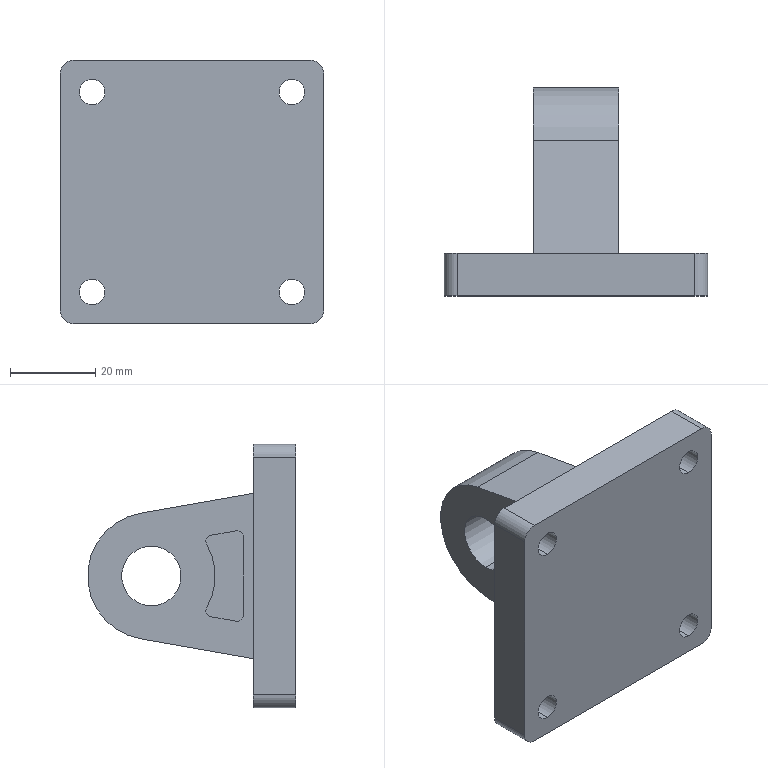Part | STEP file | 1 solid | 45 faces | box 62 x 49 x 62 mm | volume 56958 mm3 | cylinder 27 | plane 18 | commonest cylinder face diameters 2.8 x10 6 x8 6.2 x4 30 x3 14 x2